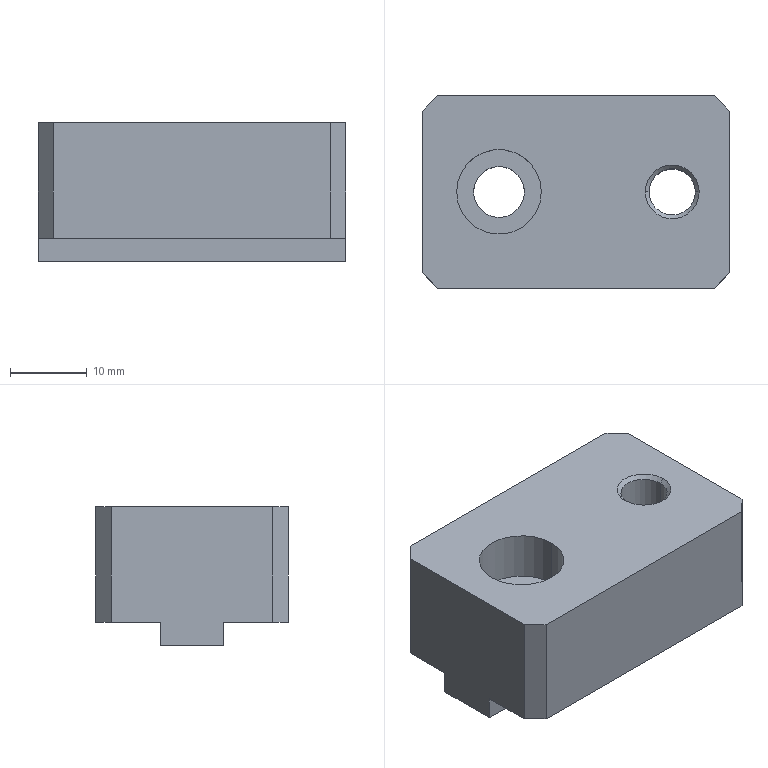Part | SolidWorks | features Chamfer 2, ICE 2, Extrusion 1, HoleWzd 1 | 1 solid | 23 faces | box 40 x 25 x 18 mm | volume 14348 mm3 | plane 15 | cylinder 6 | cone 2 | commonest cylinder face diameters 6 x2 6.6 x2 11 x2
STEP:
#1=CARTESIAN_POINT('',(29.5,12.5,14.5));
#2=VERTEX_POINT('',#1);
#3=CARTESIAN_POINT('',(35.5,12.5,14.5));
#4=VERTEX_POINT('',#3);
#5=CARTESIAN_POINT('',(32.5,12.5,14.5));
#6=DIRECTION('',(0.,0.,1.));
#7=DIRECTION('',(-1.,0.,0.));
#8=AXIS2_PLACEMENT_3D('',#5,#6,#7);
#9=CIRCLE('',#8,3.);
#10=EDGE_CURVE('',#2,#4,#9,.T.);
#11=ORIENTED_EDGE('',*,*,#10,.F.);
#12=CARTESIAN_POINT('',(29.,12.5,15.));
#13=VERTEX_POINT('',#12);
#14=CARTESIAN_POINT('',(29.5,12.5,14.5));
#15=DIRECTION('',(-0.7071,0.,0.7071));
#16=VECTOR('',#15,1000.);
#17=LINE('',#14,#16);
#18=EDGE_CURVE('',#2,#13,#17,.T.);
#19=ORIENTED_EDGE('',*,*,#18,.T.);
#20=CARTESIAN_POINT('',(36.,12.5,15.));
#21=VERTEX_POINT('',#20);
#22=CARTESIAN_POINT('',(32.5,12.5,15.));
#23=DIRECTION('',(0.,0.,-1.));
#24=DIRECTION('',(-1.,0.,0.));
#25=AXIS2_PLACEMENT_3D('',#22,#23,#24);
#26=CIRCLE('',#25,3.5);
#27=EDGE_CURVE('',#21,#13,#26,.T.);
#28=ORIENTED_EDGE('',*,*,#27,.F.);
#29=CARTESIAN_POINT('',(35.5,12.5,14.5));
#30=DIRECTION('',(0.7071,0.,0.7071));
#31=VECTOR('',#30,1000.);
#32=LINE('',#29,#31);
#33=EDGE_CURVE('',#4,#21,#32,.T.);
#34=ORIENTED_EDGE('',*,*,#33,.F.);
#35=EDGE_LOOP('',(#11,#19,#28,#34));
#36=FACE_OUTER_BOUND('',#35,.T.);
#37=CARTESIAN_POINT('',(32.5,12.5,14.5));
#38=DIRECTION('',(0.,0.,1.));
#39=DIRECTION('',(1.,0.,0.));
#40=AXIS2_PLACEMENT_3D('',#37,#38,#39);
#41=CONICAL_SURFACE('',#40,3.,0.7854);
#42=ADVANCED_FACE('',(#36),#41,.F.);
#43=CARTESIAN_POINT('',(29.5,12.5,-3.));
#44=VERTEX_POINT('',#43);
#45=CARTESIAN_POINT('',(35.5,12.5,-3.));
#46=VERTEX_POINT('',#45);
#47=CARTESIAN_POINT('',(32.5,12.5,-3.));
#48=DIRECTION('',(0.,0.,1.));
#49=DIRECTION('',(1.,0.,0.));
#50=AXIS2_PLACEMENT_3D('',#47,#48,#49);
#51=CIRCLE('',#50,3.);
#52=EDGE_CURVE('',#44,#46,#51,.T.);
#53=ORIENTED_EDGE('',*,*,#52,.F.);
#54=CARTESIAN_POINT('',(29.5,12.5,-3.));
#55=DIRECTION('',(0.,0.,1.));
#56=VECTOR('',#55,1000.);
#57=LINE('',#54,#56);
#58=EDGE_CURVE('',#44,#2,#57,.T.);
#59=ORIENTED_EDGE('',*,*,#58,.T.);
#60=ORIENTED_EDGE('',*,*,#10,.T.);
#61=CARTESIAN_POINT('',(35.5,12.5,-3.));
#62=DIRECTION('',(0.,0.,1.));
#63=VECTOR('',#62,1000.);
#64=LINE('',#61,#63);
#65=EDGE_CURVE('',#46,#4,#64,.T.);
#66=ORIENTED_EDGE('',*,*,#65,.F.);
#67=EDGE_LOOP('',(#53,#59,#60,#66));
#68=FACE_OUTER_BOUND('',#67,.T.);
#69=CARTESIAN_POINT('',(32.5,12.5,-3.));
#70=DIRECTION('',(0.,0.,1.));
#71=DIRECTION('',(1.,0.,0.));
#72=AXIS2_PLACEMENT_3D('',#69,#70,#71);
#73=CYLINDRICAL_SURFACE('',#72,3.);
#74=ADVANCED_FACE('',(#68),#73,.F.);
#75=CARTESIAN_POINT('',(4.5,12.5,8.6));
#76=VERTEX_POINT('',#75);
#77=CARTESIAN_POINT('',(15.5,12.5,8.6));
#78=VERTEX_POINT('',#77);
#79=CARTESIAN_POINT('',(10.,12.5,8.6));
#80=DIRECTION('',(0.,0.,1.));
#81=DIRECTION('',(1.,0.,0.));
#82=AXIS2_PLACEMENT_3D('',#79,#80,#81);
#83=CIRCLE('',#82,5.5);
#84=EDGE_CURVE('',#76,#78,#83,.T.);
#85=ORIENTED_EDGE('',*,*,#84,.F.);
#86=CARTESIAN_POINT('',(4.5,12.5,15.));
#87=VERTEX_POINT('',#86);
#88=CARTESIAN_POINT('',(4.5,12.5,15.));
#89=DIRECTION('',(0.,0.,1.));
#90=VECTOR('',#89,1000.);
#91=LINE('',#88,#90);
#92=EDGE_CURVE('',#76,#87,#91,.T.);
#93=ORIENTED_EDGE('',*,*,#92,.T.);
#94=CARTESIAN_POINT('',(15.5,12.5,15.));
#95=VERTEX_POINT('',#94);
#96=CARTESIAN_POINT('',(10.,12.5,15.));
#97=DIRECTION('',(0.,0.,1.));
#98=DIRECTION('',(1.,0.,0.));
#99=AXIS2_PLACEMENT_3D('',#96,#97,#98);
#100=CIRCLE('',#99,5.5);
#101=EDGE_CURVE('',#87,#95,#100,.T.);
#102=ORIENTED_EDGE('',*,*,#101,.T.);
#103=CARTESIAN_POINT('',(15.5,12.5,15.));
#104=DIRECTION('',(0.,0.,1.));
#105=VECTOR('',#104,1000.);
#106=LINE('',#103,#105);
#107=EDGE_CURVE('',#78,#95,#106,.T.);
#108=ORIENTED_EDGE('',*,*,#107,.F.);
#109=EDGE_LOOP('',(#85,#93,#102,#108));
#110=FACE_OUTER_BOUND('',#109,.T.);
#111=CARTESIAN_POINT('',(10.,12.5,15.));
#112=DIRECTION('',(0.,0.,1.));
#113=DIRECTION('',(1.,0.,0.));
#114=AXIS2_PLACEMENT_3D('',#111,#112,#113);
#115=CYLINDRICAL_SURFACE('',#114,5.5);
#116=ADVANCED_FACE('',(#110),#115,.F.);
#117=CARTESIAN_POINT('',(6.7,12.5,-3.));
#118=VERTEX_POINT('',#117);
#119=CARTESIAN_POINT('',(13.3,12.5,-3.));
#120=VERTEX_POINT('',#119);
#121=CARTESIAN_POINT('',(10.,12.5,-3.));
#122=DIRECTION('',(0.,0.,1.));
#123=DIRECTION('',(1.,0.,0.));
#124=AXIS2_PLACEMENT_3D('',#121,#122,#123);
#125=CIRCLE('',#124,3.3);
#126=EDGE_CURVE('',#118,#120,#125,.T.);
#127=ORIENTED_EDGE('',*,*,#126,.F.);
#128=CARTESIAN_POINT('',(6.7,12.5,8.6));
#129=VERTEX_POINT('',#128);
#130=CARTESIAN_POINT('',(6.7,12.5,15.));
#131=DIRECTION('',(0.,0.,1.));
#132=VECTOR('',#131,1000.);
#133=LINE('',#130,#132);
#134=EDGE_CURVE('',#118,#129,#133,.T.);
#135=ORIENTED_EDGE('',*,*,#134,.T.);
#136=CARTESIAN_POINT('',(13.3,12.5,8.6));
#137=VERTEX_POINT('',#136);
#138=CARTESIAN_POINT('',(10.,12.5,8.6));
#139=DIRECTION('',(0.,0.,1.));
#140=DIRECTION('',(1.,0.,0.));
#141=AXIS2_PLACEMENT_3D('',#138,#139,#140);
#142=CIRCLE('',#141,3.3);
#143=EDGE_CURVE('',#129,#137,#142,.T.);
#144=ORIENTED_EDGE('',*,*,#143,.T.);
#145=CARTESIAN_POINT('',(13.3,12.5,15.));
#146=DIRECTION('',(0.,0.,1.));
#147=VECTOR('',#146,1000.);
#148=LINE('',#145,#147);
#149=EDGE_CURVE('',#120,#137,#148,.T.);
#150=ORIENTED_EDGE('',*,*,#149,.F.);
#151=EDGE_LOOP('',(#127,#135,#144,#150));
#152=FACE_OUTER_BOUND('',#151,.T.);
#153=CARTESIAN_POINT('',(10.,12.5,15.));
#154=DIRECTION('',(0.,0.,1.));
#155=DIRECTION('',(1.,0.,0.));
#156=AXIS2_PLACEMENT_3D('',#153,#154,#155);
#157=CYLINDRICAL_SURFACE('',#156,3.3);
#158=ADVANCED_FACE('',(#152),#157,.F.);
#159=CARTESIAN_POINT('',(0.,23.,0.));
#160=VERTEX_POINT('',#159);
#161=CARTESIAN_POINT('',(0.,16.6,0.));
#162=VERTEX_POINT('',#161);
#163=CARTESIAN_POINT('',(0.,0.,0.));
#164=DIRECTION('',(0.,-1.,0.));
#165=VECTOR('',#164,1000.);
#166=LINE('',#163,#165);
#167=EDGE_CURVE('',#160,#162,#166,.T.);
#168=ORIENTED_EDGE('',*,*,#167,.F.);
#169=CARTESIAN_POINT('',(2.,25.,0.));
#170=VERTEX_POINT('',#169);
#171=CARTESIAN_POINT('',(-11.5,11.5,0.));
#172=DIRECTION('',(0.7071,0.7071,0.));
#173=VECTOR('',#172,1000.);
#174=LINE('',#171,#173);
#175=EDGE_CURVE('',#160,#170,#174,.T.);
#176=ORIENTED_EDGE('',*,*,#175,.T.);
#177=CARTESIAN_POINT('',(38.,25.,0.));
#178=VERTEX_POINT('',#177);
#179=CARTESIAN_POINT('',(0.,25.,0.));
#180=DIRECTION('',(-1.,0.,0.));
#181=VECTOR('',#180,1000.);
#182=LINE('',#179,#181);
#183=EDGE_CURVE('',#178,#170,#182,.T.);
#184=ORIENTED_EDGE('',*,*,#183,.F.);
#185=CARTESIAN_POINT('',(40.,23.,0.));
#186=VERTEX_POINT('',#185);
#187=CARTESIAN_POINT('',(31.5,31.5,0.));
#188=DIRECTION('',(0.7071,-0.7071,0.));
#189=VECTOR('',#188,1000.);
#190=LINE('',#187,#189);
#191=EDGE_CURVE('',#178,#186,#190,.T.);
#192=ORIENTED_EDGE('',*,*,#191,.T.);
#193=CARTESIAN_POINT('',(40.,16.6,0.));
#194=VERTEX_POINT('',#193);
#195=CARTESIAN_POINT('',(40.,0.,0.));
#196=DIRECTION('',(0.,1.,0.));
#197=VECTOR('',#196,1000.);
#198=LINE('',#195,#197);
#199=EDGE_CURVE('',#194,#186,#198,.T.);
#200=ORIENTED_EDGE('',*,*,#199,.F.);
#201=CARTESIAN_POINT('',(40.,16.6,0.));
#202=DIRECTION('',(1.,0.,0.));
#203=VECTOR('',#202,1000.);
#204=LINE('',#201,#203);
#205=EDGE_CURVE('',#162,#194,#204,.T.);
#206=ORIENTED_EDGE('',*,*,#205,.F.);
#207=EDGE_LOOP('',(#168,#176,#184,#192,#200,#206));
#208=FACE_OUTER_BOUND('',#207,.T.);
#209=CARTESIAN_POINT('',(0.,0.,0.));
#210=DIRECTION('',(0.,0.,-1.));
#211=DIRECTION('',(-1.,0.,0.));
#212=AXIS2_PLACEMENT_3D('',#209,#210,#211);
#213=PLANE('',#212);
#214=ADVANCED_FACE('',(#208),#213,.T.);
#215=CARTESIAN_POINT('',(0.,8.4,0.));
#216=VERTEX_POINT('',#215);
#217=CARTESIAN_POINT('',(0.,2.,0.));
#218=VERTEX_POINT('',#217);
#219=CARTESIAN_POINT('',(0.,0.,0.));
#220=DIRECTION('',(0.,-1.,0.));
#221=VECTOR('',#220,1000.);
#222=LINE('',#219,#221);
#223=EDGE_CURVE('',#216,#218,#222,.T.);
#224=ORIENTED_EDGE('',*,*,#223,.T.);
#225=CARTESIAN_POINT('',(0.,2.,15.));
#226=VERTEX_POINT('',#225);
#227=CARTESIAN_POINT('',(0.,2.,15.));
#228=DIRECTION('',(0.,0.,1.));
#229=VECTOR('',#228,1000.);
#230=LINE('',#227,#229);
#231=EDGE_CURVE('',#218,#226,#230,.T.);
#232=ORIENTED_EDGE('',*,*,#231,.T.);
#233=CARTESIAN_POINT('',(0.,23.,15.));
#234=VERTEX_POINT('',#233);
#235=CARTESIAN_POINT('',(0.,0.,15.));
#236=DIRECTION('',(0.,-1.,0.));
#237=VECTOR('',#236,1000.);
#238=LINE('',#235,#237);
#239=EDGE_CURVE('',#234,#226,#238,.T.);
#240=ORIENTED_EDGE('',*,*,#239,.F.);
#241=CARTESIAN_POINT('',(0.,23.,15.));
#242=DIRECTION('',(0.,0.,-1.));
#243=VECTOR('',#242,1000.);
#244=LINE('',#241,#243);
#245=EDGE_CURVE('',#234,#160,#244,.T.);
#246=ORIENTED_EDGE('',*,*,#245,.T.);
#247=ORIENTED_EDGE('',*,*,#167,.T.);
#248=CARTESIAN_POINT('',(0.,16.6,-3.));
#249=VERTEX_POINT('',#248);
#250=CARTESIAN_POINT('',(0.,16.6,-3.));
#251=DIRECTION('',(0.,0.,1.));
#252=VECTOR('',#251,1000.);
#253=LINE('',#250,#252);
#254=EDGE_CURVE('',#249,#162,#253,.T.);
#255=ORIENTED_EDGE('',*,*,#254,.F.);
#256=CARTESIAN_POINT('',(0.,8.4,-3.));
#257=VERTEX_POINT('',#256);
#258=CARTESIAN_POINT('',(0.,8.4,-3.));
#259=DIRECTION('',(0.,1.,0.));
#260=VECTOR('',#259,1000.);
#261=LINE('',#258,#260);
#262=EDGE_CURVE('',#257,#249,#261,.T.);
#263=ORIENTED_EDGE('',*,*,#262,.F.);
#264=CARTESIAN_POINT('',(0.,8.4,-3.));
#265=DIRECTION('',(0.,0.,1.));
#266=VECTOR('',#265,1000.);
#267=LINE('',#264,#266);
#268=EDGE_CURVE('',#257,#216,#267,.T.);
#269=ORIENTED_EDGE('',*,*,#268,.T.);
#270=EDGE_LOOP('',(#224,#232,#240,#246,#247,#255,#263,#269));
#271=FACE_OUTER_BOUND('',#270,.T.);
#272=CARTESIAN_POINT('',(0.,0.,15.));
#273=DIRECTION('',(1.,0.,0.));
#274=DIRECTION('',(0.,1.,0.));
#275=AXIS2_PLACEMENT_3D('',#272,#273,#274);
#276=PLANE('',#275);
#277=ADVANCED_FACE('',(#271),#276,.F.);
#278=CARTESIAN_POINT('',(2.,0.,0.));
#279=VERTEX_POINT('',#278);
#280=CARTESIAN_POINT('',(38.,0.,0.));
#281=VERTEX_POINT('',#280);
#282=CARTESIAN_POINT('',(0.,0.,0.));
#283=DIRECTION('',(1.,0.,0.));
#284=VECTOR('',#283,1000.);
#285=LINE('',#282,#284);
#286=EDGE_CURVE('',#279,#281,#285,.T.);
#287=ORIENTED_EDGE('',*,*,#286,.T.);
#288=CARTESIAN_POINT('',(38.,0.,15.));
#289=VERTEX_POINT('',#288);
#290=CARTESIAN_POINT('',(38.,0.,15.));
#291=DIRECTION('',(0.,0.,1.));
#292=VECTOR('',#291,1000.);
#293=LINE('',#290,#292);
#294=EDGE_CURVE('',#281,#289,#293,.T.);
#295=ORIENTED_EDGE('',*,*,#294,.T.);
#296=CARTESIAN_POINT('',(2.,0.,15.));
#297=VERTEX_POINT('',#296);
#298=CARTESIAN_POINT('',(0.,0.,15.));
#299=DIRECTION('',(1.,0.,0.));
#300=VECTOR('',#299,1000.);
#301=LINE('',#298,#300);
#302=EDGE_CURVE('',#297,#289,#301,.T.);
#303=ORIENTED_EDGE('',*,*,#302,.F.);
#304=CARTESIAN_POINT('',(2.,0.,15.));
#305=DIRECTION('',(0.,0.,-1.));
#306=VECTOR('',#305,1000.);
#307=LINE('',#304,#306);
#308=EDGE_CURVE('',#297,#279,#307,.T.);
#309=ORIENTED_EDGE('',*,*,#308,.T.);
#310=EDGE_LOOP('',(#287,#295,#303,#309));
#311=FACE_OUTER_BOUND('',#310,.T.);
#312=CARTESIAN_POINT('',(0.,0.,15.));
#313=DIRECTION('',(0.,1.,0.));
#314=DIRECTION('',(0.,0.,1.));
#315=AXIS2_PLACEMENT_3D('',#312,#313,#314);
#316=PLANE('',#315);
#317=ADVANCED_FACE('',(#311),#316,.F.);
#318=CARTESIAN_POINT('',(40.,2.,15.));
#319=VERTEX_POINT('',#318);
#320=CARTESIAN_POINT('',(40.,23.,15.));
#321=VERTEX_POINT('',#320);
#322=CARTESIAN_POINT('',(40.,0.,15.));
#323=DIRECTION('',(0.,1.,0.));
#324=VECTOR('',#323,1000.);
#325=LINE('',#322,#324);
#326=EDGE_CURVE('',#319,#321,#325,.T.);
#327=ORIENTED_EDGE('',*,*,#326,.F.);
#328=CARTESIAN_POINT('',(40.,2.,0.));
#329=VERTEX_POINT('',#328);
#330=CARTESIAN_POINT('',(40.,2.,15.));
#331=DIRECTION('',(0.,0.,-1.));
#332=VECTOR('',#331,1000.);
#333=LINE('',#330,#332);
#334=EDGE_CURVE('',#319,#329,#333,.T.);
#335=ORIENTED_EDGE('',*,*,#334,.T.);
#336=CARTESIAN_POINT('',(40.,8.4,0.));
#337=VERTEX_POINT('',#336);
#338=CARTESIAN_POINT('',(40.,0.,0.));
#339=DIRECTION('',(0.,1.,0.));
#340=VECTOR('',#339,1000.);
#341=LINE('',#338,#340);
#342=EDGE_CURVE('',#329,#337,#341,.T.);
#343=ORIENTED_EDGE('',*,*,#342,.T.);
#344=CARTESIAN_POINT('',(40.,8.4,-3.));
#345=VERTEX_POINT('',#344);
#346=CARTESIAN_POINT('',(40.,8.4,-3.));
#347=DIRECTION('',(0.,0.,1.));
#348=VECTOR('',#347,1000.);
#349=LINE('',#346,#348);
#350=EDGE_CURVE('',#345,#337,#349,.T.);
#351=ORIENTED_EDGE('',*,*,#350,.F.);
#352=CARTESIAN_POINT('',(40.,16.6,-3.));
#353=VERTEX_POINT('',#352);
#354=CARTESIAN_POINT('',(40.,8.4,-3.));
#355=DIRECTION('',(0.,-1.,0.));
#356=VECTOR('',#355,1000.);
#357=LINE('',#354,#356);
#358=EDGE_CURVE('',#353,#345,#357,.T.);
#359=ORIENTED_EDGE('',*,*,#358,.F.);
#360=CARTESIAN_POINT('',(40.,16.6,-3.));
#361=DIRECTION('',(0.,0.,1.));
#362=VECTOR('',#361,1000.);
#363=LINE('',#360,#362);
#364=EDGE_CURVE('',#353,#194,#363,.T.);
#365=ORIENTED_EDGE('',*,*,#364,.T.);
#366=ORIENTED_EDGE('',*,*,#199,.T.);
#367=CARTESIAN_POINT('',(40.,23.,15.));
#368=DIRECTION('',(0.,0.,1.));
#369=VECTOR('',#368,1000.);
#370=LINE('',#367,#369);
#371=EDGE_CURVE('',#186,#321,#370,.T.);
#372=ORIENTED_EDGE('',*,*,#371,.T.);
#373=EDGE_LOOP('',(#327,#335,#343,#351,#359,#365,#366,#372));
#374=FACE_OUTER_BOUND('',#373,.T.);
#375=CARTESIAN_POINT('',(40.,0.,15.));
#376=DIRECTION('',(-1.,0.,0.));
#377=DIRECTION('',(0.,0.,1.));
#378=AXIS2_PLACEMENT_3D('',#375,#376,#377);
#379=PLANE('',#378);
#380=ADVANCED_FACE('',(#374),#379,.F.);
#381=ORIENTED_EDGE('',*,*,#183,.T.);
#382=CARTESIAN_POINT('',(2.,25.,15.));
#383=VERTEX_POINT('',#382);
#384=CARTESIAN_POINT('',(2.,25.,15.));
#385=DIRECTION('',(0.,0.,1.));
#386=VECTOR('',#385,1000.);
#387=LINE('',#384,#386);
#388=EDGE_CURVE('',#170,#383,#387,.T.);
#389=ORIENTED_EDGE('',*,*,#388,.T.);
#390=CARTESIAN_POINT('',(38.,25.,15.));
#391=VERTEX_POINT('',#390);
#392=CARTESIAN_POINT('',(0.,25.,15.));
#393=DIRECTION('',(-1.,0.,0.));
#394=VECTOR('',#393,1000.);
#395=LINE('',#392,#394);
#396=EDGE_CURVE('',#391,#383,#395,.T.);
#397=ORIENTED_EDGE('',*,*,#396,.F.);
#398=CARTESIAN_POINT('',(38.,25.,15.));
#399=DIRECTION('',(0.,0.,-1.));
#400=VECTOR('',#399,1000.);
#401=LINE('',#398,#400);
#402=EDGE_CURVE('',#391,#178,#401,.T.);
#403=ORIENTED_EDGE('',*,*,#402,.T.);
#404=EDGE_LOOP('',(#381,#389,#397,#403));
#405=FACE_OUTER_BOUND('',#404,.T.);
#406=CARTESIAN_POINT('',(0.,25.,15.));
#407=DIRECTION('',(0.,-1.,0.));
#408=DIRECTION('',(0.,0.,-1.));
#409=AXIS2_PLACEMENT_3D('',#406,#407,#408);
#410=PLANE('',#409);
#411=ADVANCED_FACE('',(#405),#410,.F.);
#412=ORIENTED_EDGE('',*,*,#27,.T.);
#413=CARTESIAN_POINT('',(32.5,12.5,15.));
#414=DIRECTION('',(0.,0.,-1.));
#415=DIRECTION('',(-1.,0.,0.));
#416=AXIS2_PLACEMENT_3D('',#413,#414,#415);
#417=CIRCLE('',#416,3.5);
#418=EDGE_CURVE('',#13,#21,#417,.T.);
#419=ORIENTED_EDGE('',*,*,#418,.T.);
#420=EDGE_LOOP('',(#412,#419));
#421=FACE_BOUND('',#420,.T.);
#422=CARTESIAN_POINT('',(10.,12.5,15.));
#423=DIRECTION('',(0.,0.,1.));
#424=DIRECTION('',(1.,0.,0.));
#425=AXIS2_PLACEMENT_3D('',#422,#423,#424);
#426=CIRCLE('',#425,5.5);
#427=EDGE_CURVE('',#95,#87,#426,.T.);
#428=ORIENTED_EDGE('',*,*,#427,.F.);
#429=ORIENTED_EDGE('',*,*,#101,.F.);
#430=EDGE_LOOP('',(#428,#429));
#431=FACE_BOUND('',#430,.T.);
#432=ORIENTED_EDGE('',*,*,#302,.T.);
#433=CARTESIAN_POINT('',(40.,2.,15.));
#434=DIRECTION('',(0.7071,0.7071,0.));
#435=VECTOR('',#434,1000.);
#436=LINE('',#433,#435);
#437=EDGE_CURVE('',#289,#319,#436,.T.);
#438=ORIENTED_EDGE('',*,*,#437,.T.);
#439=ORIENTED_EDGE('',*,*,#326,.T.);
#440=CARTESIAN_POINT('',(38.,25.,15.));
#441=DIRECTION('',(-0.7071,0.7071,0.));
#442=VECTOR('',#441,1000.);
#443=LINE('',#440,#442);
#444=EDGE_CURVE('',#321,#391,#443,.T.);
#445=ORIENTED_EDGE('',*,*,#444,.T.);
#446=ORIENTED_EDGE('',*,*,#396,.T.);
#447=CARTESIAN_POINT('',(0.,23.,15.));
#448=DIRECTION('',(-0.7071,-0.7071,0.));
#449=VECTOR('',#448,1000.);
#450=LINE('',#447,#449);
#451=EDGE_CURVE('',#383,#234,#450,.T.);
#452=ORIENTED_EDGE('',*,*,#451,.T.);
#453=ORIENTED_EDGE('',*,*,#239,.T.);
#454=CARTESIAN_POINT('',(2.,0.,15.));
#455=DIRECTION('',(0.7071,-0.7071,0.));
#456=VECTOR('',#455,1000.);
#457=LINE('',#454,#456);
#458=EDGE_CURVE('',#226,#297,#457,.T.);
#459=ORIENTED_EDGE('',*,*,#458,.T.);
#460=EDGE_LOOP('',(#432,#438,#439,#445,#446,#452,#453,#459));
#461=FACE_OUTER_BOUND('',#460,.T.);
#462=CARTESIAN_POINT('',(0.,0.,15.));
#463=DIRECTION('',(0.,0.,-1.));
#464=DIRECTION('',(-1.,0.,0.));
#465=AXIS2_PLACEMENT_3D('',#462,#463,#464);
#466=PLANE('',#465);
#467=ADVANCED_FACE('',(#421,#431,#461),#466,.F.);
#468=ORIENTED_EDGE('',*,*,#342,.F.);
#469=CARTESIAN_POINT('',(19.,-19.,0.));
#470=DIRECTION('',(-0.7071,-0.7071,0.));
#471=VECTOR('',#470,1000.);
#472=LINE('',#469,#471);
#473=EDGE_CURVE('',#329,#281,#472,.T.);
#474=ORIENTED_EDGE('',*,*,#473,.T.);
#475=ORIENTED_EDGE('',*,*,#286,.F.);
#476=CARTESIAN_POINT('',(1.,1.,0.));
#477=DIRECTION('',(-0.7071,0.7071,0.));
#478=VECTOR('',#477,1000.);
#479=LINE('',#476,#478);
#480=EDGE_CURVE('',#279,#218,#479,.T.);
#481=ORIENTED_EDGE('',*,*,#480,.T.);
#482=ORIENTED_EDGE('',*,*,#223,.F.);
#483=CARTESIAN_POINT('',(40.,8.4,0.));
#484=DIRECTION('',(-1.,0.,0.));
#485=VECTOR('',#484,1000.);
#486=LINE('',#483,#485);
#487=EDGE_CURVE('',#337,#216,#486,.T.);
#488=ORIENTED_EDGE('',*,*,#487,.F.);
#489=EDGE_LOOP('',(#468,#474,#475,#481,#482,#488));
#490=FACE_OUTER_BOUND('',#489,.T.);
#491=CARTESIAN_POINT('',(0.,0.,0.));
#492=DIRECTION('',(0.,0.,-1.));
#493=DIRECTION('',(-1.,0.,0.));
#494=AXIS2_PLACEMENT_3D('',#491,#492,#493);
#495=PLANE('',#494);
#496=ADVANCED_FACE('',(#490),#495,.T.);
#497=ORIENTED_EDGE('',*,*,#487,.T.);
#498=ORIENTED_EDGE('',*,*,#268,.F.);
#499=CARTESIAN_POINT('',(40.,8.4,-3.));
#500=DIRECTION('',(-1.,0.,0.));
#501=VECTOR('',#500,1000.);
#502=LINE('',#499,#501);
#503=EDGE_CURVE('',#345,#257,#502,.T.);
#504=ORIENTED_EDGE('',*,*,#503,.F.);
#505=ORIENTED_EDGE('',*,*,#350,.T.);
#506=EDGE_LOOP('',(#497,#498,#504,#505));
#507=FACE_OUTER_BOUND('',#506,.T.);
#508=CARTESIAN_POINT('',(40.,8.4,-3.));
#509=DIRECTION('',(0.,1.,0.));
#510=DIRECTION('',(0.,0.,1.));
#511=AXIS2_PLACEMENT_3D('',#508,#509,#510);
#512=PLANE('',#511);
#513=ADVANCED_FACE('',(#507),#512,.F.);
#514=ORIENTED_EDGE('',*,*,#205,.T.);
#515=ORIENTED_EDGE('',*,*,#364,.F.);
#516=CARTESIAN_POINT('',(40.,16.6,-3.));
#517=DIRECTION('',(1.,0.,0.));
#518=VECTOR('',#517,1000.);
#519=LINE('',#516,#518);
#520=EDGE_CURVE('',#249,#353,#519,.T.);
#521=ORIENTED_EDGE('',*,*,#520,.F.);
#522=ORIENTED_EDGE('',*,*,#254,.T.);
#523=EDGE_LOOP('',(#514,#515,#521,#522));
#524=FACE_OUTER_BOUND('',#523,.T.);
#525=CARTESIAN_POINT('',(40.,16.6,-3.));
#526=DIRECTION('',(0.,-1.,0.));
#527=DIRECTION('',(1.,0.,0.));
#528=AXIS2_PLACEMENT_3D('',#525,#526,#527);
#529=PLANE('',#528);
#530=ADVANCED_FACE('',(#524),#529,.F.);
#531=CARTESIAN_POINT('',(32.5,12.5,-3.));
#532=DIRECTION('',(0.,0.,1.));
#533=DIRECTION('',(1.,0.,0.));
#534=AXIS2_PLACEMENT_3D('',#531,#532,#533);
#535=CIRCLE('',#534,3.);
#536=EDGE_CURVE('',#46,#44,#535,.T.);
#537=ORIENTED_EDGE('',*,*,#536,.T.);
#538=ORIENTED_EDGE('',*,*,#52,.T.);
#539=EDGE_LOOP('',(#537,#538));
#540=FACE_BOUND('',#539,.T.);
#541=CARTESIAN_POINT('',(10.,12.5,-3.));
#542=DIRECTION('',(0.,0.,1.));
#543=DIRECTION('',(1.,0.,0.));
#544=AXIS2_PLACEMENT_3D('',#541,#542,#543);
#545=CIRCLE('',#544,3.3);
#546=EDGE_CURVE('',#120,#118,#545,.T.);
#547=ORIENTED_EDGE('',*,*,#546,.T.);
#548=ORIENTED_EDGE('',*,*,#126,.T.);
#549=EDGE_LOOP('',(#547,#548));
#550=FACE_BOUND('',#549,.T.);
#551=ORIENTED_EDGE('',*,*,#358,.T.);
#552=ORIENTED_EDGE('',*,*,#503,.T.);
#553=ORIENTED_EDGE('',*,*,#262,.T.);
#554=ORIENTED_EDGE('',*,*,#520,.T.);
#555=EDGE_LOOP('',(#551,#552,#553,#554));
#556=FACE_OUTER_BOUND('',#555,.T.);
#557=CARTESIAN_POINT('',(0.,0.,-3.));
#558=DIRECTION('',(0.,0.,1.));
#559=DIRECTION('',(1.,0.,0.));
#560=AXIS2_PLACEMENT_3D('',#557,#558,#559);
#561=PLANE('',#560);
#562=ADVANCED_FACE('',(#540,#550,#556),#561,.F.);
#563=ORIENTED_EDGE('',*,*,#134,.F.);
#564=ORIENTED_EDGE('',*,*,#546,.F.);
#565=ORIENTED_EDGE('',*,*,#149,.T.);
#566=CARTESIAN_POINT('',(10.,12.5,8.6));
#567=DIRECTION('',(0.,0.,1.));
#568=DIRECTION('',(1.,0.,0.));
#569=AXIS2_PLACEMENT_3D('',#566,#567,#568);
#570=CIRCLE('',#569,3.3);
#571=EDGE_CURVE('',#137,#129,#570,.T.);
#572=ORIENTED_EDGE('',*,*,#571,.T.);
#573=EDGE_LOOP('',(#563,#564,#565,#572));
#574=FACE_OUTER_BOUND('',#573,.T.);
#575=CARTESIAN_POINT('',(10.,12.5,15.));
#576=DIRECTION('',(0.,0.,1.));
#577=DIRECTION('',(1.,0.,0.));
#578=AXIS2_PLACEMENT_3D('',#575,#576,#577);
#579=CYLINDRICAL_SURFACE('',#578,3.3);
#580=ADVANCED_FACE('',(#574),#579,.F.);
#581=ORIENTED_EDGE('',*,*,#571,.F.);
#582=ORIENTED_EDGE('',*,*,#143,.F.);
#583=EDGE_LOOP('',(#581,#582));
#584=FACE_BOUND('',#583,.T.);
#585=CARTESIAN_POINT('',(10.,12.5,8.6));
#586=DIRECTION('',(0.,0.,1.));
#587=DIRECTION('',(1.,0.,0.));
#588=AXIS2_PLACEMENT_3D('',#585,#586,#587);
#589=CIRCLE('',#588,5.5);
#590=EDGE_CURVE('',#78,#76,#589,.T.);
#591=ORIENTED_EDGE('',*,*,#590,.T.);
#592=ORIENTED_EDGE('',*,*,#84,.T.);
#593=EDGE_LOOP('',(#591,#592));
#594=FACE_OUTER_BOUND('',#593,.T.);
#595=CARTESIAN_POINT('',(13.3,12.5,8.6));
#596=DIRECTION('',(0.,0.,-1.));
#597=DIRECTION('',(-1.,0.,0.));
#598=AXIS2_PLACEMENT_3D('',#595,#596,#597);
#599=PLANE('',#598);
#600=ADVANCED_FACE('',(#584,#594),#599,.F.);
#601=ORIENTED_EDGE('',*,*,#92,.F.);
#602=ORIENTED_EDGE('',*,*,#590,.F.);
#603=ORIENTED_EDGE('',*,*,#107,.T.);
#604=ORIENTED_EDGE('',*,*,#427,.T.);
#605=EDGE_LOOP('',(#601,#602,#603,#604));
#606=FACE_OUTER_BOUND('',#605,.T.);
#607=CARTESIAN_POINT('',(10.,12.5,15.));
#608=DIRECTION('',(0.,0.,1.));
#609=DIRECTION('',(1.,0.,0.));
#610=AXIS2_PLACEMENT_3D('',#607,#608,#609);
#611=CYLINDRICAL_SURFACE('',#610,5.5);
#612=ADVANCED_FACE('',(#606),#611,.F.);
#613=ORIENTED_EDGE('',*,*,#58,.F.);
#614=ORIENTED_EDGE('',*,*,#536,.F.);
#615=ORIENTED_EDGE('',*,*,#65,.T.);
#616=CARTESIAN_POINT('',(32.5,12.5,14.5));
#617=DIRECTION('',(0.,0.,1.));
#618=DIRECTION('',(-1.,0.,0.));
#619=AXIS2_PLACEMENT_3D('',#616,#617,#618);
#620=CIRCLE('',#619,3.);
#621=EDGE_CURVE('',#4,#2,#620,.T.);
#622=ORIENTED_EDGE('',*,*,#621,.T.);
#623=EDGE_LOOP('',(#613,#614,#615,#622));
#624=FACE_OUTER_BOUND('',#623,.T.);
#625=CARTESIAN_POINT('',(32.5,12.5,-3.));
#626=DIRECTION('',(0.,0.,1.));
#627=DIRECTION('',(1.,0.,0.));
#628=AXIS2_PLACEMENT_3D('',#625,#626,#627);
#629=CYLINDRICAL_SURFACE('',#628,3.);
#630=ADVANCED_FACE('',(#624),#629,.F.);
#631=ORIENTED_EDGE('',*,*,#18,.F.);
#632=ORIENTED_EDGE('',*,*,#621,.F.);
#633=ORIENTED_EDGE('',*,*,#33,.T.);
#634=ORIENTED_EDGE('',*,*,#418,.F.);
#635=EDGE_LOOP('',(#631,#632,#633,#634));
#636=FACE_OUTER_BOUND('',#635,.T.);
#637=CARTESIAN_POINT('',(32.5,12.5,14.5));
#638=DIRECTION('',(0.,0.,1.));
#639=DIRECTION('',(1.,0.,0.));
#640=AXIS2_PLACEMENT_3D('',#637,#638,#639);
#641=CONICAL_SURFACE('',#640,3.,0.7854);
#642=ADVANCED_FACE('',(#636),#641,.F.);
#643=ORIENTED_EDGE('',*,*,#437,.F.);
#644=ORIENTED_EDGE('',*,*,#294,.F.);
#645=ORIENTED_EDGE('',*,*,#473,.F.);
#646=ORIENTED_EDGE('',*,*,#334,.F.);
#647=EDGE_LOOP('',(#643,#644,#645,#646));
#648=FACE_OUTER_BOUND('',#647,.T.);
#649=CARTESIAN_POINT('',(40.,2.,15.));
#650=DIRECTION('',(-0.7071,0.7071,0.));
#651=DIRECTION('',(0.,0.,-1.));
#652=AXIS2_PLACEMENT_3D('',#649,#650,#651);
#653=PLANE('',#652);
#654=ADVANCED_FACE('',(#648),#653,.F.);
#655=ORIENTED_EDGE('',*,*,#458,.F.);
#656=ORIENTED_EDGE('',*,*,#231,.F.);
#657=ORIENTED_EDGE('',*,*,#480,.F.);
#658=ORIENTED_EDGE('',*,*,#308,.F.);
#659=EDGE_LOOP('',(#655,#656,#657,#658));
#660=FACE_OUTER_BOUND('',#659,.T.);
#661=CARTESIAN_POINT('',(2.,0.,15.));
#662=DIRECTION('',(0.7071,0.7071,0.));
#663=DIRECTION('',(0.,0.,-1.));
#664=AXIS2_PLACEMENT_3D('',#661,#662,#663);
#665=PLANE('',#664);
#666=ADVANCED_FACE('',(#660),#665,.F.);
#667=ORIENTED_EDGE('',*,*,#451,.F.);
#668=ORIENTED_EDGE('',*,*,#388,.F.);
#669=ORIENTED_EDGE('',*,*,#175,.F.);
#670=ORIENTED_EDGE('',*,*,#245,.F.);
#671=EDGE_LOOP('',(#667,#668,#669,#670));
#672=FACE_OUTER_BOUND('',#671,.T.);
#673=CARTESIAN_POINT('',(0.,23.,15.));
#674=DIRECTION('',(0.7071,-0.7071,0.));
#675=DIRECTION('',(0.,0.,-1.));
#676=AXIS2_PLACEMENT_3D('',#673,#674,#675);
#677=PLANE('',#676);
#678=ADVANCED_FACE('',(#672),#677,.F.);
#679=ORIENTED_EDGE('',*,*,#444,.F.);
#680=ORIENTED_EDGE('',*,*,#371,.F.);
#681=ORIENTED_EDGE('',*,*,#191,.F.);
#682=ORIENTED_EDGE('',*,*,#402,.F.);
#683=EDGE_LOOP('',(#679,#680,#681,#682));
#684=FACE_OUTER_BOUND('',#683,.T.);
#685=CARTESIAN_POINT('',(38.,25.,15.));
#686=DIRECTION('',(-0.7071,-0.7071,0.));
#687=DIRECTION('',(0.,0.,-1.));
#688=AXIS2_PLACEMENT_3D('',#685,#686,#687);
#689=PLANE('',#688);
#690=ADVANCED_FACE('',(#684),#689,.F.);
#691=CLOSED_SHELL('',(#42,#74,#116,#158,#214,#277,#317,#380,#411,#467,#496,#513,#530,#562,#580,#600,#612,#630,#642,#654,#666,#678,#690));
#692=MANIFOLD_SOLID_BREP('',#691);
#693=CARTESIAN_POINT('',(0.,0.,0.));
#694=DIRECTION('',(0.,0.,1.));
#695=DIRECTION('',(1.,0.,0.));
#696=AXIS2_PLACEMENT_3D('',#693,#694,#695);
#697=(LENGTH_UNIT()NAMED_UNIT(*)SI_UNIT(.MILLI.,.METRE.));
#698=UNCERTAINTY_MEASURE_WITH_UNIT(LENGTH_MEASURE(0.00001),#697,'','');
#699=(NAMED_UNIT(*)PLANE_ANGLE_UNIT()SI_UNIT($,.RADIAN.));
#700=(NAMED_UNIT(*)SI_UNIT($,.STERADIAN.)SOLID_ANGLE_UNIT());
#701=(GEOMETRIC_REPRESENTATION_CONTEXT(3)GLOBAL_UNCERTAINTY_ASSIGNED_CONTEXT((#698))GLOBAL_UNIT_ASSIGNED_CONTEXT((#697,#699,#700))REPRESENTATION_CONTEXT('',''));
#702=ADVANCED_BREP_SHAPE_REPRESENTATION('',(#692,#696),#701);